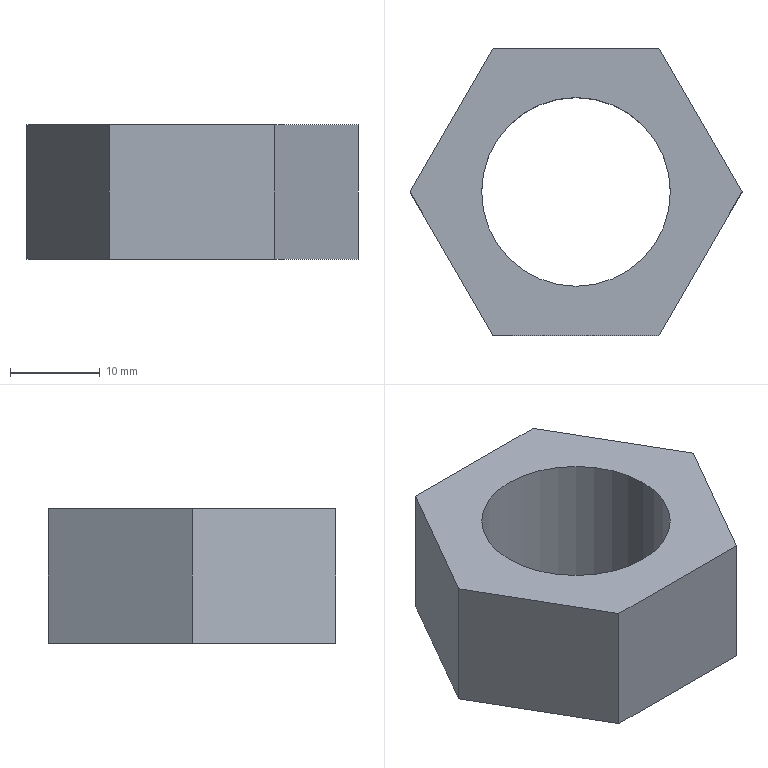Part | SolidWorks | features Extrusion 1, HoleWzd 1 | 1 solid | 10 faces | box 36.95 x 32 x 15 mm | volume 8107 mm3 | plane 8 | cylinder 2 | commonest cylinder face diameters 21 x2
STEP:
#1=CARTESIAN_POINT('',(-10.5,0.,0.));
#2=VERTEX_POINT('',#1);
#3=CARTESIAN_POINT('',(10.5,0.,0.));
#4=VERTEX_POINT('',#3);
#5=CARTESIAN_POINT('',(0.,0.,0.));
#6=DIRECTION('',(0.,0.,1.));
#7=DIRECTION('',(1.,0.,0.));
#8=AXIS2_PLACEMENT_3D('',#5,#6,#7);
#9=CIRCLE('',#8,10.5);
#10=EDGE_CURVE('',#2,#4,#9,.T.);
#11=ORIENTED_EDGE('',*,*,#10,.F.);
#12=CARTESIAN_POINT('',(-10.5,0.,15.));
#13=VERTEX_POINT('',#12);
#14=CARTESIAN_POINT('',(-10.5,0.,15.));
#15=DIRECTION('',(0.,0.,1.));
#16=VECTOR('',#15,1000.);
#17=LINE('',#14,#16);
#18=EDGE_CURVE('',#2,#13,#17,.T.);
#19=ORIENTED_EDGE('',*,*,#18,.T.);
#20=CARTESIAN_POINT('',(10.5,0.,15.));
#21=VERTEX_POINT('',#20);
#22=CARTESIAN_POINT('',(0.,0.,15.));
#23=DIRECTION('',(0.,0.,1.));
#24=DIRECTION('',(1.,0.,0.));
#25=AXIS2_PLACEMENT_3D('',#22,#23,#24);
#26=CIRCLE('',#25,10.5);
#27=EDGE_CURVE('',#13,#21,#26,.T.);
#28=ORIENTED_EDGE('',*,*,#27,.T.);
#29=CARTESIAN_POINT('',(10.5,0.,15.));
#30=DIRECTION('',(0.,0.,1.));
#31=VECTOR('',#30,1000.);
#32=LINE('',#29,#31);
#33=EDGE_CURVE('',#4,#21,#32,.T.);
#34=ORIENTED_EDGE('',*,*,#33,.F.);
#35=EDGE_LOOP('',(#11,#19,#28,#34));
#36=FACE_OUTER_BOUND('',#35,.T.);
#37=CARTESIAN_POINT('',(0.,0.,15.));
#38=DIRECTION('',(0.,0.,1.));
#39=DIRECTION('',(1.,0.,0.));
#40=AXIS2_PLACEMENT_3D('',#37,#38,#39);
#41=CYLINDRICAL_SURFACE('',#40,10.5);
#42=ADVANCED_FACE('',(#36),#41,.F.);
#43=CARTESIAN_POINT('',(9.238,-16.,0.));
#44=VERTEX_POINT('',#43);
#45=CARTESIAN_POINT('',(18.475,0.,0.));
#46=VERTEX_POINT('',#45);
#47=CARTESIAN_POINT('',(9.238,-16.,0.));
#48=DIRECTION('',(0.5,0.866,0.));
#49=VECTOR('',#48,1000.);
#50=LINE('',#47,#49);
#51=EDGE_CURVE('',#44,#46,#50,.T.);
#52=ORIENTED_EDGE('',*,*,#51,.T.);
#53=CARTESIAN_POINT('',(18.475,0.,15.));
#54=VERTEX_POINT('',#53);
#55=CARTESIAN_POINT('',(18.475,0.,15.));
#56=DIRECTION('',(0.,0.,-1.));
#57=VECTOR('',#56,1000.);
#58=LINE('',#55,#57);
#59=EDGE_CURVE('',#54,#46,#58,.T.);
#60=ORIENTED_EDGE('',*,*,#59,.F.);
#61=CARTESIAN_POINT('',(9.238,-16.,15.));
#62=VERTEX_POINT('',#61);
#63=CARTESIAN_POINT('',(9.238,-16.,15.));
#64=DIRECTION('',(0.5,0.866,0.));
#65=VECTOR('',#64,1000.);
#66=LINE('',#63,#65);
#67=EDGE_CURVE('',#62,#54,#66,.T.);
#68=ORIENTED_EDGE('',*,*,#67,.F.);
#69=CARTESIAN_POINT('',(9.238,-16.,15.));
#70=DIRECTION('',(0.,0.,-1.));
#71=VECTOR('',#70,1000.);
#72=LINE('',#69,#71);
#73=EDGE_CURVE('',#62,#44,#72,.T.);
#74=ORIENTED_EDGE('',*,*,#73,.T.);
#75=EDGE_LOOP('',(#52,#60,#68,#74));
#76=FACE_OUTER_BOUND('',#75,.T.);
#77=CARTESIAN_POINT('',(9.238,-16.,15.));
#78=DIRECTION('',(-0.866,0.5,0.));
#79=DIRECTION('',(-0.5,-0.866,0.));
#80=AXIS2_PLACEMENT_3D('',#77,#78,#79);
#81=PLANE('',#80);
#82=ADVANCED_FACE('',(#76),#81,.F.);
#83=CARTESIAN_POINT('',(9.238,16.,0.));
#84=VERTEX_POINT('',#83);
#85=CARTESIAN_POINT('',(18.475,0.,0.));
#86=DIRECTION('',(-0.5,0.866,0.));
#87=VECTOR('',#86,1000.);
#88=LINE('',#85,#87);
#89=EDGE_CURVE('',#46,#84,#88,.T.);
#90=ORIENTED_EDGE('',*,*,#89,.T.);
#91=CARTESIAN_POINT('',(9.238,16.,15.));
#92=VERTEX_POINT('',#91);
#93=CARTESIAN_POINT('',(9.238,16.,15.));
#94=DIRECTION('',(0.,0.,-1.));
#95=VECTOR('',#94,1000.);
#96=LINE('',#93,#95);
#97=EDGE_CURVE('',#92,#84,#96,.T.);
#98=ORIENTED_EDGE('',*,*,#97,.F.);
#99=CARTESIAN_POINT('',(18.475,0.,15.));
#100=DIRECTION('',(-0.5,0.866,0.));
#101=VECTOR('',#100,1000.);
#102=LINE('',#99,#101);
#103=EDGE_CURVE('',#54,#92,#102,.T.);
#104=ORIENTED_EDGE('',*,*,#103,.F.);
#105=ORIENTED_EDGE('',*,*,#59,.T.);
#106=EDGE_LOOP('',(#90,#98,#104,#105));
#107=FACE_OUTER_BOUND('',#106,.T.);
#108=CARTESIAN_POINT('',(18.475,0.,15.));
#109=DIRECTION('',(-0.866,-0.5,0.));
#110=DIRECTION('',(0.5,-0.866,0.));
#111=AXIS2_PLACEMENT_3D('',#108,#109,#110);
#112=PLANE('',#111);
#113=ADVANCED_FACE('',(#107),#112,.F.);
#114=CARTESIAN_POINT('',(-9.238,16.,0.));
#115=VERTEX_POINT('',#114);
#116=CARTESIAN_POINT('',(9.238,16.,0.));
#117=DIRECTION('',(-1.,0.,0.));
#118=VECTOR('',#117,1000.);
#119=LINE('',#116,#118);
#120=EDGE_CURVE('',#84,#115,#119,.T.);
#121=ORIENTED_EDGE('',*,*,#120,.T.);
#122=CARTESIAN_POINT('',(-9.238,16.,15.));
#123=VERTEX_POINT('',#122);
#124=CARTESIAN_POINT('',(-9.238,16.,15.));
#125=DIRECTION('',(0.,0.,-1.));
#126=VECTOR('',#125,1000.);
#127=LINE('',#124,#126);
#128=EDGE_CURVE('',#123,#115,#127,.T.);
#129=ORIENTED_EDGE('',*,*,#128,.F.);
#130=CARTESIAN_POINT('',(9.238,16.,15.));
#131=DIRECTION('',(-1.,0.,0.));
#132=VECTOR('',#131,1000.);
#133=LINE('',#130,#132);
#134=EDGE_CURVE('',#92,#123,#133,.T.);
#135=ORIENTED_EDGE('',*,*,#134,.F.);
#136=ORIENTED_EDGE('',*,*,#97,.T.);
#137=EDGE_LOOP('',(#121,#129,#135,#136));
#138=FACE_OUTER_BOUND('',#137,.T.);
#139=CARTESIAN_POINT('',(9.238,16.,15.));
#140=DIRECTION('',(0.,-1.,0.));
#141=DIRECTION('',(0.,0.,-1.));
#142=AXIS2_PLACEMENT_3D('',#139,#140,#141);
#143=PLANE('',#142);
#144=ADVANCED_FACE('',(#138),#143,.F.);
#145=CARTESIAN_POINT('',(-18.475,0.,0.));
#146=VERTEX_POINT('',#145);
#147=CARTESIAN_POINT('',(-9.238,16.,0.));
#148=DIRECTION('',(-0.5,-0.866,0.));
#149=VECTOR('',#148,1000.);
#150=LINE('',#147,#149);
#151=EDGE_CURVE('',#115,#146,#150,.T.);
#152=ORIENTED_EDGE('',*,*,#151,.T.);
#153=CARTESIAN_POINT('',(-18.475,0.,15.));
#154=VERTEX_POINT('',#153);
#155=CARTESIAN_POINT('',(-18.475,0.,15.));
#156=DIRECTION('',(0.,0.,-1.));
#157=VECTOR('',#156,1000.);
#158=LINE('',#155,#157);
#159=EDGE_CURVE('',#154,#146,#158,.T.);
#160=ORIENTED_EDGE('',*,*,#159,.F.);
#161=CARTESIAN_POINT('',(-9.238,16.,15.));
#162=DIRECTION('',(-0.5,-0.866,0.));
#163=VECTOR('',#162,1000.);
#164=LINE('',#161,#163);
#165=EDGE_CURVE('',#123,#154,#164,.T.);
#166=ORIENTED_EDGE('',*,*,#165,.F.);
#167=ORIENTED_EDGE('',*,*,#128,.T.);
#168=EDGE_LOOP('',(#152,#160,#166,#167));
#169=FACE_OUTER_BOUND('',#168,.T.);
#170=CARTESIAN_POINT('',(-9.238,16.,15.));
#171=DIRECTION('',(0.866,-0.5,0.));
#172=DIRECTION('',(0.5,0.866,0.));
#173=AXIS2_PLACEMENT_3D('',#170,#171,#172);
#174=PLANE('',#173);
#175=ADVANCED_FACE('',(#169),#174,.F.);
#176=CARTESIAN_POINT('',(-9.238,-16.,0.));
#177=VERTEX_POINT('',#176);
#178=CARTESIAN_POINT('',(-18.475,0.,0.));
#179=DIRECTION('',(0.5,-0.866,0.));
#180=VECTOR('',#179,1000.);
#181=LINE('',#178,#180);
#182=EDGE_CURVE('',#146,#177,#181,.T.);
#183=ORIENTED_EDGE('',*,*,#182,.T.);
#184=CARTESIAN_POINT('',(-9.238,-16.,15.));
#185=VERTEX_POINT('',#184);
#186=CARTESIAN_POINT('',(-9.238,-16.,15.));
#187=DIRECTION('',(0.,0.,-1.));
#188=VECTOR('',#187,1000.);
#189=LINE('',#186,#188);
#190=EDGE_CURVE('',#185,#177,#189,.T.);
#191=ORIENTED_EDGE('',*,*,#190,.F.);
#192=CARTESIAN_POINT('',(-18.475,0.,15.));
#193=DIRECTION('',(0.5,-0.866,0.));
#194=VECTOR('',#193,1000.);
#195=LINE('',#192,#194);
#196=EDGE_CURVE('',#154,#185,#195,.T.);
#197=ORIENTED_EDGE('',*,*,#196,.F.);
#198=ORIENTED_EDGE('',*,*,#159,.T.);
#199=EDGE_LOOP('',(#183,#191,#197,#198));
#200=FACE_OUTER_BOUND('',#199,.T.);
#201=CARTESIAN_POINT('',(-18.475,0.,15.));
#202=DIRECTION('',(0.866,0.5,0.));
#203=DIRECTION('',(-0.5,0.866,0.));
#204=AXIS2_PLACEMENT_3D('',#201,#202,#203);
#205=PLANE('',#204);
#206=ADVANCED_FACE('',(#200),#205,.F.);
#207=CARTESIAN_POINT('',(-9.238,-16.,0.));
#208=DIRECTION('',(1.,0.,0.));
#209=VECTOR('',#208,1000.);
#210=LINE('',#207,#209);
#211=EDGE_CURVE('',#177,#44,#210,.T.);
#212=ORIENTED_EDGE('',*,*,#211,.T.);
#213=ORIENTED_EDGE('',*,*,#73,.F.);
#214=CARTESIAN_POINT('',(-9.238,-16.,15.));
#215=DIRECTION('',(1.,0.,0.));
#216=VECTOR('',#215,1000.);
#217=LINE('',#214,#216);
#218=EDGE_CURVE('',#185,#62,#217,.T.);
#219=ORIENTED_EDGE('',*,*,#218,.F.);
#220=ORIENTED_EDGE('',*,*,#190,.T.);
#221=EDGE_LOOP('',(#212,#213,#219,#220));
#222=FACE_OUTER_BOUND('',#221,.T.);
#223=CARTESIAN_POINT('',(-9.238,-16.,15.));
#224=DIRECTION('',(0.,1.,0.));
#225=DIRECTION('',(0.,0.,1.));
#226=AXIS2_PLACEMENT_3D('',#223,#224,#225);
#227=PLANE('',#226);
#228=ADVANCED_FACE('',(#222),#227,.F.);
#229=CARTESIAN_POINT('',(0.,0.,15.));
#230=DIRECTION('',(0.,0.,1.));
#231=DIRECTION('',(1.,0.,0.));
#232=AXIS2_PLACEMENT_3D('',#229,#230,#231);
#233=CIRCLE('',#232,10.5);
#234=EDGE_CURVE('',#21,#13,#233,.T.);
#235=ORIENTED_EDGE('',*,*,#234,.F.);
#236=ORIENTED_EDGE('',*,*,#27,.F.);
#237=EDGE_LOOP('',(#235,#236));
#238=FACE_BOUND('',#237,.T.);
#239=ORIENTED_EDGE('',*,*,#67,.T.);
#240=ORIENTED_EDGE('',*,*,#103,.T.);
#241=ORIENTED_EDGE('',*,*,#134,.T.);
#242=ORIENTED_EDGE('',*,*,#165,.T.);
#243=ORIENTED_EDGE('',*,*,#196,.T.);
#244=ORIENTED_EDGE('',*,*,#218,.T.);
#245=EDGE_LOOP('',(#239,#240,#241,#242,#243,#244));
#246=FACE_OUTER_BOUND('',#245,.T.);
#247=CARTESIAN_POINT('',(18.475,0.,15.));
#248=DIRECTION('',(0.,0.,1.));
#249=DIRECTION('',(1.,0.,0.));
#250=AXIS2_PLACEMENT_3D('',#247,#248,#249);
#251=PLANE('',#250);
#252=ADVANCED_FACE('',(#238,#246),#251,.T.);
#253=CARTESIAN_POINT('',(0.,0.,0.));
#254=DIRECTION('',(0.,0.,1.));
#255=DIRECTION('',(1.,0.,0.));
#256=AXIS2_PLACEMENT_3D('',#253,#254,#255);
#257=CIRCLE('',#256,10.5);
#258=EDGE_CURVE('',#4,#2,#257,.T.);
#259=ORIENTED_EDGE('',*,*,#258,.T.);
#260=ORIENTED_EDGE('',*,*,#10,.T.);
#261=EDGE_LOOP('',(#259,#260));
#262=FACE_BOUND('',#261,.T.);
#263=ORIENTED_EDGE('',*,*,#51,.F.);
#264=ORIENTED_EDGE('',*,*,#211,.F.);
#265=ORIENTED_EDGE('',*,*,#182,.F.);
#266=ORIENTED_EDGE('',*,*,#151,.F.);
#267=ORIENTED_EDGE('',*,*,#120,.F.);
#268=ORIENTED_EDGE('',*,*,#89,.F.);
#269=EDGE_LOOP('',(#263,#264,#265,#266,#267,#268));
#270=FACE_OUTER_BOUND('',#269,.T.);
#271=CARTESIAN_POINT('',(18.475,0.,0.));
#272=DIRECTION('',(0.,0.,1.));
#273=DIRECTION('',(1.,0.,0.));
#274=AXIS2_PLACEMENT_3D('',#271,#272,#273);
#275=PLANE('',#274);
#276=ADVANCED_FACE('',(#262,#270),#275,.F.);
#277=ORIENTED_EDGE('',*,*,#18,.F.);
#278=ORIENTED_EDGE('',*,*,#258,.F.);
#279=ORIENTED_EDGE('',*,*,#33,.T.);
#280=ORIENTED_EDGE('',*,*,#234,.T.);
#281=EDGE_LOOP('',(#277,#278,#279,#280));
#282=FACE_OUTER_BOUND('',#281,.T.);
#283=CARTESIAN_POINT('',(0.,0.,15.));
#284=DIRECTION('',(0.,0.,1.));
#285=DIRECTION('',(1.,0.,0.));
#286=AXIS2_PLACEMENT_3D('',#283,#284,#285);
#287=CYLINDRICAL_SURFACE('',#286,10.5);
#288=ADVANCED_FACE('',(#282),#287,.F.);
#289=CLOSED_SHELL('',(#42,#82,#113,#144,#175,#206,#228,#252,#276,#288));
#290=MANIFOLD_SOLID_BREP('',#289);
#291=CARTESIAN_POINT('',(0.,0.,0.));
#292=DIRECTION('',(0.,0.,1.));
#293=DIRECTION('',(1.,0.,0.));
#294=AXIS2_PLACEMENT_3D('',#291,#292,#293);
#295=(LENGTH_UNIT()NAMED_UNIT(*)SI_UNIT(.MILLI.,.METRE.));
#296=UNCERTAINTY_MEASURE_WITH_UNIT(LENGTH_MEASURE(0.00001),#295,'','');
#297=(NAMED_UNIT(*)PLANE_ANGLE_UNIT()SI_UNIT($,.RADIAN.));
#298=(NAMED_UNIT(*)SI_UNIT($,.STERADIAN.)SOLID_ANGLE_UNIT());
#299=(GEOMETRIC_REPRESENTATION_CONTEXT(3)GLOBAL_UNCERTAINTY_ASSIGNED_CONTEXT((#296))GLOBAL_UNIT_ASSIGNED_CONTEXT((#295,#297,#298))REPRESENTATION_CONTEXT('',''));
#300=ADVANCED_BREP_SHAPE_REPRESENTATION('',(#290,#294),#299);